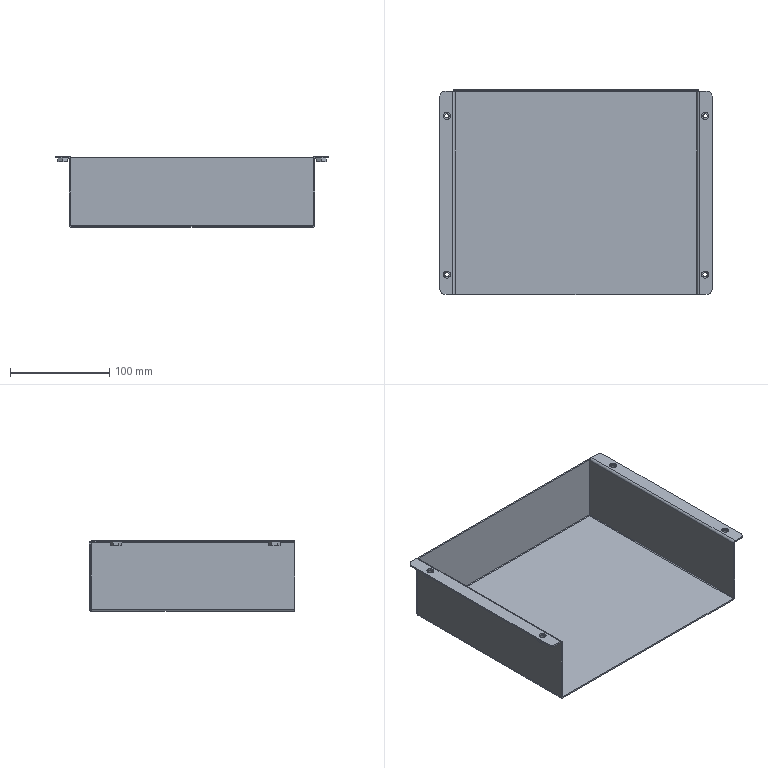Part | SolidWorks | features BaseBody 5 | 5 solids | 88 faces | box 274 x 206.5 x 71.5 mm | volume 153067 mm3 | plane 54 | cylinder 30 | spline 4 | commonest cylinder face diameters 4.2 x8 7.1 x8 1.473 x5 4.473 x5 10 x4